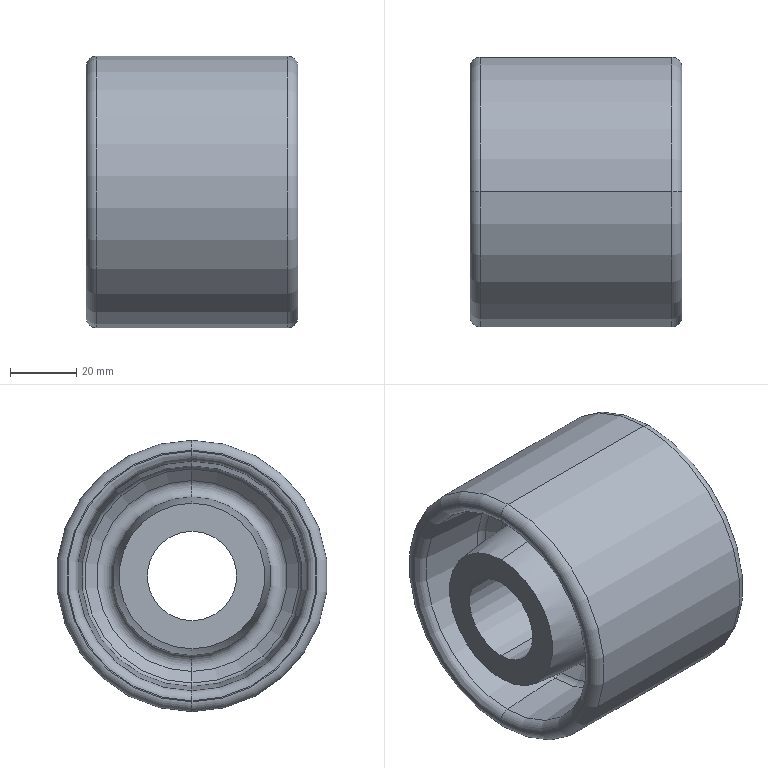Part | SolidWorks | features Revolution 1 | 1 solid | 36 faces | box 64 x 82 x 82 mm | volume 200004 mm3 | torus 24 | cone 4 | plane 4 | cylinder 4 | commonest cylinder face diameters 27 x2 82 x2
STEP:
#1=CARTESIAN_POINT('',(-32.713,0.,48.22));
#2=VERTEX_POINT('',#1);
#3=CARTESIAN_POINT('',(-32.713,0.,-21.22));
#4=VERTEX_POINT('',#3);
#5=CARTESIAN_POINT('',(-32.713,0.,13.5));
#6=DIRECTION('',(-1.,0.,0.));
#7=DIRECTION('',(0.,0.,1.));
#8=AXIS2_PLACEMENT_3D('',#5,#6,#7);
#9=CIRCLE('',#8,34.72);
#10=EDGE_CURVE('',#2,#4,#9,.T.);
#11=ORIENTED_EDGE('',*,*,#10,.T.);
#12=CARTESIAN_POINT('',(-12.328,0.,-19.908));
#13=VERTEX_POINT('',#12);
#14=CARTESIAN_POINT('',(-3.418,0.,-317.446));
#15=DIRECTION('',(0.,1.,0.));
#16=DIRECTION('',(0.,0.,1.));
#17=AXIS2_PLACEMENT_3D('',#14,#15,#16);
#18=CIRCLE('',#17,297.671);
#19=EDGE_CURVE('',#4,#13,#18,.T.);
#20=ORIENTED_EDGE('',*,*,#19,.T.);
#21=CARTESIAN_POINT('',(-12.328,0.,46.908));
#22=VERTEX_POINT('',#21);
#23=CARTESIAN_POINT('',(-12.328,0.,13.5));
#24=DIRECTION('',(-1.,0.,0.));
#25=DIRECTION('',(0.,0.,1.));
#26=AXIS2_PLACEMENT_3D('',#23,#24,#25);
#27=CIRCLE('',#26,33.408);
#28=EDGE_CURVE('',#22,#13,#27,.T.);
#29=ORIENTED_EDGE('',*,*,#28,.F.);
#30=CARTESIAN_POINT('',(-3.418,0.,344.446));
#31=DIRECTION('',(0.,-1.,0.));
#32=DIRECTION('',(0.,0.,-1.));
#33=AXIS2_PLACEMENT_3D('',#30,#31,#32);
#34=CIRCLE('',#33,297.671);
#35=EDGE_CURVE('',#2,#22,#34,.T.);
#36=ORIENTED_EDGE('',*,*,#35,.F.);
#37=EDGE_LOOP('',(#11,#20,#29,#36));
#38=FACE_OUTER_BOUND('',#37,.T.);
#39=CARTESIAN_POINT('',(-3.418,0.,13.5));
#40=DIRECTION('',(-1.,0.,0.));
#41=DIRECTION('',(0.,0.,1.));
#42=AXIS2_PLACEMENT_3D('',#39,#40,#41);
#43=TOROIDAL_SURFACE('',#42,330.946,297.671);
#44=ADVANCED_FACE('',(#38),#43,.T.);
#45=CARTESIAN_POINT('',(-35.418,0.,51.205));
#46=VERTEX_POINT('',#45);
#47=CARTESIAN_POINT('',(-35.418,0.,-24.205));
#48=VERTEX_POINT('',#47);
#49=CARTESIAN_POINT('',(-35.418,0.,13.5));
#50=DIRECTION('',(-1.,0.,0.));
#51=DIRECTION('',(0.,0.,1.));
#52=AXIS2_PLACEMENT_3D('',#49,#50,#51);
#53=CIRCLE('',#52,37.705);
#54=EDGE_CURVE('',#46,#48,#53,.T.);
#55=ORIENTED_EDGE('',*,*,#54,.T.);
#56=CARTESIAN_POINT('',(-32.418,0.,-24.205));
#57=DIRECTION('',(0.,1.,0.));
#58=DIRECTION('',(0.,0.,1.));
#59=AXIS2_PLACEMENT_3D('',#56,#57,#58);
#60=CIRCLE('',#59,3.);
#61=EDGE_CURVE('',#48,#4,#60,.T.);
#62=ORIENTED_EDGE('',*,*,#61,.T.);
#63=ORIENTED_EDGE('',*,*,#10,.F.);
#64=CARTESIAN_POINT('',(-32.418,0.,51.205));
#65=DIRECTION('',(0.,-1.,0.));
#66=DIRECTION('',(0.,0.,-1.));
#67=AXIS2_PLACEMENT_3D('',#64,#65,#66);
#68=CIRCLE('',#67,3.);
#69=EDGE_CURVE('',#46,#2,#68,.T.);
#70=ORIENTED_EDGE('',*,*,#69,.F.);
#71=EDGE_LOOP('',(#55,#62,#63,#70));
#72=FACE_OUTER_BOUND('',#71,.T.);
#73=CARTESIAN_POINT('',(-32.418,0.,13.5));
#74=DIRECTION('',(-1.,0.,0.));
#75=DIRECTION('',(0.,0.,1.));
#76=AXIS2_PLACEMENT_3D('',#73,#74,#75);
#77=TOROIDAL_SURFACE('',#76,37.705,3.);
#78=ADVANCED_FACE('',(#72),#77,.T.);
#79=CARTESIAN_POINT('',(-32.418,0.,54.5));
#80=VERTEX_POINT('',#79);
#81=CARTESIAN_POINT('',(-32.418,0.,-27.5));
#82=VERTEX_POINT('',#81);
#83=CARTESIAN_POINT('',(-32.418,0.,13.5));
#84=DIRECTION('',(-1.,0.,0.));
#85=DIRECTION('',(0.,0.,1.));
#86=AXIS2_PLACEMENT_3D('',#83,#84,#85);
#87=CIRCLE('',#86,41.);
#88=EDGE_CURVE('',#80,#82,#87,.T.);
#89=ORIENTED_EDGE('',*,*,#88,.T.);
#90=CARTESIAN_POINT('',(-35.418,0.,-24.5));
#91=VERTEX_POINT('',#90);
#92=CARTESIAN_POINT('',(-32.418,0.,-24.5));
#93=DIRECTION('',(0.,1.,0.));
#94=DIRECTION('',(0.,0.,1.));
#95=AXIS2_PLACEMENT_3D('',#92,#93,#94);
#96=CIRCLE('',#95,3.);
#97=EDGE_CURVE('',#82,#91,#96,.T.);
#98=ORIENTED_EDGE('',*,*,#97,.T.);
#99=CARTESIAN_POINT('',(-35.418,0.,51.5));
#100=VERTEX_POINT('',#99);
#101=CARTESIAN_POINT('',(-35.418,0.,13.5));
#102=DIRECTION('',(-1.,0.,0.));
#103=DIRECTION('',(0.,0.,1.));
#104=AXIS2_PLACEMENT_3D('',#101,#102,#103);
#105=CIRCLE('',#104,38.);
#106=EDGE_CURVE('',#100,#91,#105,.T.);
#107=ORIENTED_EDGE('',*,*,#106,.F.);
#108=CARTESIAN_POINT('',(-32.418,0.,51.5));
#109=DIRECTION('',(0.,-1.,0.));
#110=DIRECTION('',(0.,0.,-1.));
#111=AXIS2_PLACEMENT_3D('',#108,#109,#110);
#112=CIRCLE('',#111,3.);
#113=EDGE_CURVE('',#80,#100,#112,.T.);
#114=ORIENTED_EDGE('',*,*,#113,.F.);
#115=EDGE_LOOP('',(#89,#98,#107,#114));
#116=FACE_OUTER_BOUND('',#115,.T.);
#117=CARTESIAN_POINT('',(-32.418,0.,13.5));
#118=DIRECTION('',(-1.,0.,0.));
#119=DIRECTION('',(0.,0.,1.));
#120=AXIS2_PLACEMENT_3D('',#117,#118,#119);
#121=TOROIDAL_SURFACE('',#120,38.,3.);
#122=ADVANCED_FACE('',(#116),#121,.T.);
#123=CARTESIAN_POINT('',(25.582,0.,54.5));
#124=VERTEX_POINT('',#123);
#125=CARTESIAN_POINT('',(25.582,0.,-27.5));
#126=VERTEX_POINT('',#125);
#127=CARTESIAN_POINT('',(25.582,0.,13.5));
#128=DIRECTION('',(-1.,0.,0.));
#129=DIRECTION('',(0.,0.,1.));
#130=AXIS2_PLACEMENT_3D('',#127,#128,#129);
#131=CIRCLE('',#130,41.);
#132=EDGE_CURVE('',#124,#126,#131,.T.);
#133=ORIENTED_EDGE('',*,*,#132,.T.);
#134=CARTESIAN_POINT('',(-39.429,0.,-27.5));
#135=DIRECTION('',(-1.,0.,0.));
#136=VECTOR('',#135,1000.);
#137=LINE('',#134,#136);
#138=EDGE_CURVE('',#126,#82,#137,.T.);
#139=ORIENTED_EDGE('',*,*,#138,.T.);
#140=ORIENTED_EDGE('',*,*,#88,.F.);
#141=CARTESIAN_POINT('',(-39.429,0.,54.5));
#142=DIRECTION('',(-1.,0.,0.));
#143=VECTOR('',#142,1000.);
#144=LINE('',#141,#143);
#145=EDGE_CURVE('',#124,#80,#144,.T.);
#146=ORIENTED_EDGE('',*,*,#145,.F.);
#147=EDGE_LOOP('',(#133,#139,#140,#146));
#148=FACE_OUTER_BOUND('',#147,.T.);
#149=CARTESIAN_POINT('',(-39.429,0.,13.5));
#150=DIRECTION('',(-1.,0.,0.));
#151=DIRECTION('',(0.,0.,1.));
#152=AXIS2_PLACEMENT_3D('',#149,#150,#151);
#153=CYLINDRICAL_SURFACE('',#152,41.);
#154=ADVANCED_FACE('',(#148),#153,.T.);
#155=CARTESIAN_POINT('',(28.582,0.,51.5));
#156=VERTEX_POINT('',#155);
#157=CARTESIAN_POINT('',(28.582,0.,-24.5));
#158=VERTEX_POINT('',#157);
#159=CARTESIAN_POINT('',(28.582,0.,13.5));
#160=DIRECTION('',(-1.,0.,0.));
#161=DIRECTION('',(0.,0.,1.));
#162=AXIS2_PLACEMENT_3D('',#159,#160,#161);
#163=CIRCLE('',#162,38.);
#164=EDGE_CURVE('',#156,#158,#163,.T.);
#165=ORIENTED_EDGE('',*,*,#164,.T.);
#166=CARTESIAN_POINT('',(25.582,0.,-24.5));
#167=DIRECTION('',(0.,1.,0.));
#168=DIRECTION('',(0.,0.,1.));
#169=AXIS2_PLACEMENT_3D('',#166,#167,#168);
#170=CIRCLE('',#169,3.);
#171=EDGE_CURVE('',#158,#126,#170,.T.);
#172=ORIENTED_EDGE('',*,*,#171,.T.);
#173=ORIENTED_EDGE('',*,*,#132,.F.);
#174=CARTESIAN_POINT('',(25.582,0.,51.5));
#175=DIRECTION('',(0.,-1.,0.));
#176=DIRECTION('',(0.,0.,-1.));
#177=AXIS2_PLACEMENT_3D('',#174,#175,#176);
#178=CIRCLE('',#177,3.);
#179=EDGE_CURVE('',#156,#124,#178,.T.);
#180=ORIENTED_EDGE('',*,*,#179,.F.);
#181=EDGE_LOOP('',(#165,#172,#173,#180));
#182=FACE_OUTER_BOUND('',#181,.T.);
#183=CARTESIAN_POINT('',(25.582,0.,13.5));
#184=DIRECTION('',(-1.,0.,0.));
#185=DIRECTION('',(0.,0.,1.));
#186=AXIS2_PLACEMENT_3D('',#183,#184,#185);
#187=TOROIDAL_SURFACE('',#186,38.,3.);
#188=ADVANCED_FACE('',(#182),#187,.T.);
#189=CARTESIAN_POINT('',(25.877,0.,48.22));
#190=VERTEX_POINT('',#189);
#191=CARTESIAN_POINT('',(25.877,0.,-21.22));
#192=VERTEX_POINT('',#191);
#193=CARTESIAN_POINT('',(25.877,0.,13.5));
#194=DIRECTION('',(-1.,0.,0.));
#195=DIRECTION('',(0.,0.,1.));
#196=AXIS2_PLACEMENT_3D('',#193,#194,#195);
#197=CIRCLE('',#196,34.72);
#198=EDGE_CURVE('',#190,#192,#197,.T.);
#199=ORIENTED_EDGE('',*,*,#198,.T.);
#200=CARTESIAN_POINT('',(28.582,0.,-24.205));
#201=VERTEX_POINT('',#200);
#202=CARTESIAN_POINT('',(25.582,0.,-24.205));
#203=DIRECTION('',(0.,1.,0.));
#204=DIRECTION('',(0.,0.,1.));
#205=AXIS2_PLACEMENT_3D('',#202,#203,#204);
#206=CIRCLE('',#205,3.);
#207=EDGE_CURVE('',#192,#201,#206,.T.);
#208=ORIENTED_EDGE('',*,*,#207,.T.);
#209=CARTESIAN_POINT('',(28.582,0.,51.205));
#210=VERTEX_POINT('',#209);
#211=CARTESIAN_POINT('',(28.582,0.,13.5));
#212=DIRECTION('',(-1.,0.,0.));
#213=DIRECTION('',(0.,0.,1.));
#214=AXIS2_PLACEMENT_3D('',#211,#212,#213);
#215=CIRCLE('',#214,37.705);
#216=EDGE_CURVE('',#210,#201,#215,.T.);
#217=ORIENTED_EDGE('',*,*,#216,.F.);
#218=CARTESIAN_POINT('',(25.582,0.,51.205));
#219=DIRECTION('',(0.,-1.,0.));
#220=DIRECTION('',(0.,0.,-1.));
#221=AXIS2_PLACEMENT_3D('',#218,#219,#220);
#222=CIRCLE('',#221,3.);
#223=EDGE_CURVE('',#190,#210,#222,.T.);
#224=ORIENTED_EDGE('',*,*,#223,.F.);
#225=EDGE_LOOP('',(#199,#208,#217,#224));
#226=FACE_OUTER_BOUND('',#225,.T.);
#227=CARTESIAN_POINT('',(25.582,0.,13.5));
#228=DIRECTION('',(-1.,0.,0.));
#229=DIRECTION('',(0.,0.,1.));
#230=AXIS2_PLACEMENT_3D('',#227,#228,#229);
#231=TOROIDAL_SURFACE('',#230,37.705,3.);
#232=ADVANCED_FACE('',(#226),#231,.T.);
#233=CARTESIAN_POINT('',(5.492,0.,46.908));
#234=VERTEX_POINT('',#233);
#235=CARTESIAN_POINT('',(5.492,0.,-19.908));
#236=VERTEX_POINT('',#235);
#237=CARTESIAN_POINT('',(5.492,0.,13.5));
#238=DIRECTION('',(-1.,0.,0.));
#239=DIRECTION('',(0.,0.,1.));
#240=AXIS2_PLACEMENT_3D('',#237,#238,#239);
#241=CIRCLE('',#240,33.408);
#242=EDGE_CURVE('',#234,#236,#241,.T.);
#243=ORIENTED_EDGE('',*,*,#242,.T.);
#244=CARTESIAN_POINT('',(-3.418,0.,-317.446));
#245=DIRECTION('',(0.,1.,0.));
#246=DIRECTION('',(0.,0.,1.));
#247=AXIS2_PLACEMENT_3D('',#244,#245,#246);
#248=CIRCLE('',#247,297.671);
#249=EDGE_CURVE('',#236,#192,#248,.T.);
#250=ORIENTED_EDGE('',*,*,#249,.T.);
#251=ORIENTED_EDGE('',*,*,#198,.F.);
#252=CARTESIAN_POINT('',(-3.418,0.,344.446));
#253=DIRECTION('',(0.,-1.,0.));
#254=DIRECTION('',(0.,0.,-1.));
#255=AXIS2_PLACEMENT_3D('',#252,#253,#254);
#256=CIRCLE('',#255,297.671);
#257=EDGE_CURVE('',#234,#190,#256,.T.);
#258=ORIENTED_EDGE('',*,*,#257,.F.);
#259=EDGE_LOOP('',(#243,#250,#251,#258));
#260=FACE_OUTER_BOUND('',#259,.T.);
#261=CARTESIAN_POINT('',(-3.418,0.,13.5));
#262=DIRECTION('',(-1.,0.,0.));
#263=DIRECTION('',(0.,0.,1.));
#264=AXIS2_PLACEMENT_3D('',#261,#262,#263);
#265=TOROIDAL_SURFACE('',#264,330.946,297.671);
#266=ADVANCED_FACE('',(#260),#265,.T.);
#267=CARTESIAN_POINT('',(5.492,0.,13.5));
#268=DIRECTION('',(-1.,0.,0.));
#269=DIRECTION('',(0.,0.,1.));
#270=AXIS2_PLACEMENT_3D('',#267,#268,#269);
#271=CIRCLE('',#270,33.408);
#272=EDGE_CURVE('',#236,#234,#271,.T.);
#273=ORIENTED_EDGE('',*,*,#272,.F.);
#274=CARTESIAN_POINT('',(3.298,0.,-14.965));
#275=VERTEX_POINT('',#274);
#276=CARTESIAN_POINT('',(5.582,0.,-16.91));
#277=DIRECTION('',(0.,1.,0.));
#278=DIRECTION('',(0.,0.,1.));
#279=AXIS2_PLACEMENT_3D('',#276,#277,#278);
#280=CIRCLE('',#279,3.);
#281=EDGE_CURVE('',#236,#275,#280,.T.);
#282=ORIENTED_EDGE('',*,*,#281,.T.);
#283=CARTESIAN_POINT('',(3.298,0.,41.965));
#284=VERTEX_POINT('',#283);
#285=CARTESIAN_POINT('',(3.298,0.,13.5));
#286=DIRECTION('',(-1.,0.,0.));
#287=DIRECTION('',(0.,0.,1.));
#288=AXIS2_PLACEMENT_3D('',#285,#286,#287);
#289=CIRCLE('',#288,28.465);
#290=EDGE_CURVE('',#275,#284,#289,.T.);
#291=ORIENTED_EDGE('',*,*,#290,.T.);
#292=CARTESIAN_POINT('',(5.582,0.,43.91));
#293=DIRECTION('',(0.,-1.,0.));
#294=DIRECTION('',(0.,0.,-1.));
#295=AXIS2_PLACEMENT_3D('',#292,#293,#294);
#296=CIRCLE('',#295,3.);
#297=EDGE_CURVE('',#234,#284,#296,.T.);
#298=ORIENTED_EDGE('',*,*,#297,.F.);
#299=EDGE_LOOP('',(#273,#282,#291,#298));
#300=FACE_OUTER_BOUND('',#299,.T.);
#301=CARTESIAN_POINT('',(5.582,0.,13.5));
#302=DIRECTION('',(-1.,0.,0.));
#303=DIRECTION('',(0.,0.,1.));
#304=AXIS2_PLACEMENT_3D('',#301,#302,#303);
#305=TOROIDAL_SURFACE('',#304,30.41,3.);
#306=ADVANCED_FACE('',(#300),#305,.F.);
#307=CARTESIAN_POINT('',(6.298,0.,38.442));
#308=VERTEX_POINT('',#307);
#309=CARTESIAN_POINT('',(6.298,0.,-11.442));
#310=VERTEX_POINT('',#309);
#311=CARTESIAN_POINT('',(6.298,0.,13.5));
#312=DIRECTION('',(-1.,0.,0.));
#313=DIRECTION('',(0.,0.,1.));
#314=AXIS2_PLACEMENT_3D('',#311,#312,#313);
#315=CIRCLE('',#314,24.942);
#316=EDGE_CURVE('',#308,#310,#315,.T.);
#317=ORIENTED_EDGE('',*,*,#316,.T.);
#318=CARTESIAN_POINT('',(6.298,0.,-11.442));
#319=DIRECTION('',(-0.6484,0.,-0.7613));
#320=VECTOR('',#319,1000.);
#321=LINE('',#318,#320);
#322=EDGE_CURVE('',#310,#275,#321,.T.);
#323=ORIENTED_EDGE('',*,*,#322,.T.);
#324=CARTESIAN_POINT('',(3.298,0.,13.5));
#325=DIRECTION('',(-1.,0.,0.));
#326=DIRECTION('',(0.,0.,1.));
#327=AXIS2_PLACEMENT_3D('',#324,#325,#326);
#328=CIRCLE('',#327,28.465);
#329=EDGE_CURVE('',#284,#275,#328,.T.);
#330=ORIENTED_EDGE('',*,*,#329,.F.);
#331=CARTESIAN_POINT('',(6.298,0.,38.442));
#332=DIRECTION('',(-0.6484,0.,0.7613));
#333=VECTOR('',#332,1000.);
#334=LINE('',#331,#333);
#335=EDGE_CURVE('',#308,#284,#334,.T.);
#336=ORIENTED_EDGE('',*,*,#335,.F.);
#337=EDGE_LOOP('',(#317,#323,#330,#336));
#338=FACE_OUTER_BOUND('',#337,.T.);
#339=CARTESIAN_POINT('',(6.298,0.,13.5));
#340=DIRECTION('',(-1.,0.,0.));
#341=DIRECTION('',(0.,0.,1.));
#342=AXIS2_PLACEMENT_3D('',#339,#340,#341);
#343=CONICAL_SURFACE('',#342,24.942,0.8653);
#344=ADVANCED_FACE('',(#338),#343,.T.);
#345=CARTESIAN_POINT('',(6.298,0.,13.5));
#346=DIRECTION('',(-1.,0.,0.));
#347=DIRECTION('',(0.,0.,1.));
#348=AXIS2_PLACEMENT_3D('',#345,#346,#347);
#349=CIRCLE('',#348,24.942);
#350=EDGE_CURVE('',#310,#308,#349,.T.);
#351=ORIENTED_EDGE('',*,*,#350,.F.);
#352=CARTESIAN_POINT('',(8.494,0.,-10.388));
#353=VERTEX_POINT('',#352);
#354=CARTESIAN_POINT('',(8.582,0.,-13.387));
#355=DIRECTION('',(0.,1.,0.));
#356=DIRECTION('',(0.,0.,1.));
#357=AXIS2_PLACEMENT_3D('',#354,#355,#356);
#358=CIRCLE('',#357,3.);
#359=EDGE_CURVE('',#310,#353,#358,.T.);
#360=ORIENTED_EDGE('',*,*,#359,.T.);
#361=CARTESIAN_POINT('',(8.494,0.,37.388));
#362=VERTEX_POINT('',#361);
#363=CARTESIAN_POINT('',(8.494,0.,13.5));
#364=DIRECTION('',(-1.,0.,0.));
#365=DIRECTION('',(0.,0.,1.));
#366=AXIS2_PLACEMENT_3D('',#363,#364,#365);
#367=CIRCLE('',#366,23.888);
#368=EDGE_CURVE('',#353,#362,#367,.T.);
#369=ORIENTED_EDGE('',*,*,#368,.T.);
#370=CARTESIAN_POINT('',(8.582,0.,40.387));
#371=DIRECTION('',(0.,-1.,0.));
#372=DIRECTION('',(0.,0.,-1.));
#373=AXIS2_PLACEMENT_3D('',#370,#371,#372);
#374=CIRCLE('',#373,3.);
#375=EDGE_CURVE('',#308,#362,#374,.T.);
#376=ORIENTED_EDGE('',*,*,#375,.F.);
#377=EDGE_LOOP('',(#351,#360,#369,#376));
#378=FACE_OUTER_BOUND('',#377,.T.);
#379=CARTESIAN_POINT('',(8.582,0.,13.5));
#380=DIRECTION('',(-1.,0.,0.));
#381=DIRECTION('',(0.,0.,1.));
#382=AXIS2_PLACEMENT_3D('',#379,#380,#381);
#383=TOROIDAL_SURFACE('',#382,26.887,3.);
#384=ADVANCED_FACE('',(#378),#383,.F.);
#385=CARTESIAN_POINT('',(28.582,0.,36.134));
#386=VERTEX_POINT('',#385);
#387=CARTESIAN_POINT('',(28.582,0.,-9.134));
#388=VERTEX_POINT('',#387);
#389=CARTESIAN_POINT('',(28.582,0.,13.5));
#390=DIRECTION('',(-1.,0.,0.));
#391=DIRECTION('',(0.,0.,1.));
#392=AXIS2_PLACEMENT_3D('',#389,#390,#391);
#393=CIRCLE('',#392,22.634);
#394=EDGE_CURVE('',#386,#388,#393,.T.);
#395=ORIENTED_EDGE('',*,*,#394,.T.);
#396=CARTESIAN_POINT('',(-0.4182,0.,293.862));
#397=DIRECTION('',(0.,1.,0.));
#398=DIRECTION('',(0.,0.,1.));
#399=AXIS2_PLACEMENT_3D('',#396,#397,#398);
#400=CIRCLE('',#399,304.381);
#401=EDGE_CURVE('',#388,#353,#400,.T.);
#402=ORIENTED_EDGE('',*,*,#401,.T.);
#403=CARTESIAN_POINT('',(8.494,0.,13.5));
#404=DIRECTION('',(-1.,0.,0.));
#405=DIRECTION('',(0.,0.,1.));
#406=AXIS2_PLACEMENT_3D('',#403,#404,#405);
#407=CIRCLE('',#406,23.888);
#408=EDGE_CURVE('',#362,#353,#407,.T.);
#409=ORIENTED_EDGE('',*,*,#408,.F.);
#410=CARTESIAN_POINT('',(-0.4182,0.,-266.862));
#411=DIRECTION('',(0.,-1.,0.));
#412=DIRECTION('',(0.,0.,-1.));
#413=AXIS2_PLACEMENT_3D('',#410,#411,#412);
#414=CIRCLE('',#413,304.381);
#415=EDGE_CURVE('',#386,#362,#414,.T.);
#416=ORIENTED_EDGE('',*,*,#415,.F.);
#417=EDGE_LOOP('',(#395,#402,#409,#416));
#418=FACE_OUTER_BOUND('',#417,.T.);
#419=CARTESIAN_POINT('',(-0.4182,0.,13.5));
#420=DIRECTION('',(-1.,0.,0.));
#421=DIRECTION('',(0.,0.,1.));
#422=AXIS2_PLACEMENT_3D('',#419,#420,#421);
#423=TOROIDAL_SURFACE('',#422,-280.362,304.381);
#424=ADVANCED_FACE('',(#418),#423,.T.);
#425=CARTESIAN_POINT('',(28.582,0.,0.));
#426=VERTEX_POINT('',#425);
#427=CARTESIAN_POINT('',(28.582,0.,27.));
#428=VERTEX_POINT('',#427);
#429=CARTESIAN_POINT('',(28.582,0.,13.5));
#430=DIRECTION('',(-1.,0.,0.));
#431=DIRECTION('',(0.,0.,1.));
#432=AXIS2_PLACEMENT_3D('',#429,#430,#431);
#433=CIRCLE('',#432,13.5);
#434=EDGE_CURVE('',#426,#428,#433,.T.);
#435=ORIENTED_EDGE('',*,*,#434,.F.);
#436=CARTESIAN_POINT('',(-35.418,0.,0.));
#437=VERTEX_POINT('',#436);
#438=CARTESIAN_POINT('',(-39.429,0.,0.));
#439=DIRECTION('',(-1.,0.,0.));
#440=VECTOR('',#439,1000.);
#441=LINE('',#438,#440);
#442=EDGE_CURVE('',#426,#437,#441,.T.);
#443=ORIENTED_EDGE('',*,*,#442,.T.);
#444=CARTESIAN_POINT('',(-35.418,0.,27.));
#445=VERTEX_POINT('',#444);
#446=CARTESIAN_POINT('',(-35.418,0.,13.5));
#447=DIRECTION('',(-1.,0.,0.));
#448=DIRECTION('',(0.,0.,1.));
#449=AXIS2_PLACEMENT_3D('',#446,#447,#448);
#450=CIRCLE('',#449,13.5);
#451=EDGE_CURVE('',#437,#445,#450,.T.);
#452=ORIENTED_EDGE('',*,*,#451,.T.);
#453=CARTESIAN_POINT('',(-39.429,0.,27.));
#454=DIRECTION('',(-1.,0.,0.));
#455=VECTOR('',#454,1000.);
#456=LINE('',#453,#455);
#457=EDGE_CURVE('',#428,#445,#456,.T.);
#458=ORIENTED_EDGE('',*,*,#457,.F.);
#459=EDGE_LOOP('',(#435,#443,#452,#458));
#460=FACE_OUTER_BOUND('',#459,.T.);
#461=CARTESIAN_POINT('',(-39.429,0.,13.5));
#462=DIRECTION('',(-1.,0.,0.));
#463=DIRECTION('',(0.,0.,1.));
#464=AXIS2_PLACEMENT_3D('',#461,#462,#463);
#465=CYLINDRICAL_SURFACE('',#464,13.5);
#466=ADVANCED_FACE('',(#460),#465,.F.);
#467=CARTESIAN_POINT('',(-9.33,0.,37.388));
#468=VERTEX_POINT('',#467);
#469=CARTESIAN_POINT('',(-9.33,0.,-10.388));
#470=VERTEX_POINT('',#469);
#471=CARTESIAN_POINT('',(-9.33,0.,13.5));
#472=DIRECTION('',(-1.,0.,0.));
#473=DIRECTION('',(0.,0.,1.));
#474=AXIS2_PLACEMENT_3D('',#471,#472,#473);
#475=CIRCLE('',#474,23.888);
#476=EDGE_CURVE('',#468,#470,#475,.T.);
#477=ORIENTED_EDGE('',*,*,#476,.T.);
#478=CARTESIAN_POINT('',(-35.418,0.,-8.5));
#479=VERTEX_POINT('',#478);
#480=CARTESIAN_POINT('',(-0.4182,0.,293.862));
#481=DIRECTION('',(0.,1.,0.));
#482=DIRECTION('',(0.,0.,1.));
#483=AXIS2_PLACEMENT_3D('',#480,#481,#482);
#484=CIRCLE('',#483,304.381);
#485=EDGE_CURVE('',#470,#479,#484,.T.);
#486=ORIENTED_EDGE('',*,*,#485,.T.);
#487=CARTESIAN_POINT('',(-35.418,0.,35.5));
#488=VERTEX_POINT('',#487);
#489=CARTESIAN_POINT('',(-35.418,0.,13.5));
#490=DIRECTION('',(-1.,0.,0.));
#491=DIRECTION('',(0.,0.,1.));
#492=AXIS2_PLACEMENT_3D('',#489,#490,#491);
#493=CIRCLE('',#492,22.);
#494=EDGE_CURVE('',#488,#479,#493,.T.);
#495=ORIENTED_EDGE('',*,*,#494,.F.);
#496=CARTESIAN_POINT('',(-0.4182,0.,-266.862));
#497=DIRECTION('',(0.,-1.,0.));
#498=DIRECTION('',(0.,0.,-1.));
#499=AXIS2_PLACEMENT_3D('',#496,#497,#498);
#500=CIRCLE('',#499,304.381);
#501=EDGE_CURVE('',#468,#488,#500,.T.);
#502=ORIENTED_EDGE('',*,*,#501,.F.);
#503=EDGE_LOOP('',(#477,#486,#495,#502));
#504=FACE_OUTER_BOUND('',#503,.T.);
#505=CARTESIAN_POINT('',(-0.4182,0.,13.5));
#506=DIRECTION('',(-1.,0.,0.));
#507=DIRECTION('',(0.,0.,1.));
#508=AXIS2_PLACEMENT_3D('',#505,#506,#507);
#509=TOROIDAL_SURFACE('',#508,-280.362,304.381);
#510=ADVANCED_FACE('',(#504),#509,.T.);
#511=CARTESIAN_POINT('',(-9.33,0.,13.5));
#512=DIRECTION('',(-1.,0.,0.));
#513=DIRECTION('',(0.,0.,1.));
#514=AXIS2_PLACEMENT_3D('',#511,#512,#513);
#515=CIRCLE('',#514,23.888);
#516=EDGE_CURVE('',#470,#468,#515,.T.);
#517=ORIENTED_EDGE('',*,*,#516,.F.);
#518=CARTESIAN_POINT('',(-7.134,0.,-15.332));
#519=VERTEX_POINT('',#518);
#520=CARTESIAN_POINT('',(-9.418,0.,-13.387));
#521=DIRECTION('',(0.,1.,0.));
#522=DIRECTION('',(0.,0.,1.));
#523=AXIS2_PLACEMENT_3D('',#520,#521,#522);
#524=CIRCLE('',#523,3.);
#525=EDGE_CURVE('',#470,#519,#524,.T.);
#526=ORIENTED_EDGE('',*,*,#525,.T.);
#527=CARTESIAN_POINT('',(-7.134,0.,42.332));
#528=VERTEX_POINT('',#527);
#529=CARTESIAN_POINT('',(-7.134,0.,13.5));
#530=DIRECTION('',(-1.,0.,0.));
#531=DIRECTION('',(0.,0.,1.));
#532=AXIS2_PLACEMENT_3D('',#529,#530,#531);
#533=CIRCLE('',#532,28.832);
#534=EDGE_CURVE('',#519,#528,#533,.T.);
#535=ORIENTED_EDGE('',*,*,#534,.T.);
#536=CARTESIAN_POINT('',(-9.418,0.,40.387));
#537=DIRECTION('',(0.,-1.,0.));
#538=DIRECTION('',(0.,0.,-1.));
#539=AXIS2_PLACEMENT_3D('',#536,#537,#538);
#540=CIRCLE('',#539,3.);
#541=EDGE_CURVE('',#468,#528,#540,.T.);
#542=ORIENTED_EDGE('',*,*,#541,.F.);
#543=EDGE_LOOP('',(#517,#526,#535,#542));
#544=FACE_OUTER_BOUND('',#543,.T.);
#545=CARTESIAN_POINT('',(-9.418,0.,13.5));
#546=DIRECTION('',(-1.,0.,0.));
#547=DIRECTION('',(0.,0.,1.));
#548=AXIS2_PLACEMENT_3D('',#545,#546,#547);
#549=TOROIDAL_SURFACE('',#548,26.887,3.);
#550=ADVANCED_FACE('',(#544),#549,.F.);
#551=ORIENTED_EDGE('',*,*,#534,.F.);
#552=CARTESIAN_POINT('',(-10.134,0.,-18.855));
#553=VERTEX_POINT('',#552);
#554=CARTESIAN_POINT('',(-10.134,0.,-18.855));
#555=DIRECTION('',(-0.6484,0.,-0.7613));
#556=VECTOR('',#555,1000.);
#557=LINE('',#554,#556);
#558=EDGE_CURVE('',#519,#553,#557,.T.);
#559=ORIENTED_EDGE('',*,*,#558,.T.);
#560=CARTESIAN_POINT('',(-10.134,0.,45.855));
#561=VERTEX_POINT('',#560);
#562=CARTESIAN_POINT('',(-10.134,0.,13.5));
#563=DIRECTION('',(-1.,0.,0.));
#564=DIRECTION('',(0.,0.,1.));
#565=AXIS2_PLACEMENT_3D('',#562,#563,#564);
#566=CIRCLE('',#565,32.355);
#567=EDGE_CURVE('',#553,#561,#566,.T.);
#568=ORIENTED_EDGE('',*,*,#567,.T.);
#569=CARTESIAN_POINT('',(-10.134,0.,45.855));
#570=DIRECTION('',(-0.6484,0.,0.7613));
#571=VECTOR('',#570,1000.);
#572=LINE('',#569,#571);
#573=EDGE_CURVE('',#528,#561,#572,.T.);
#574=ORIENTED_EDGE('',*,*,#573,.F.);
#575=EDGE_LOOP('',(#551,#559,#568,#574));
#576=FACE_OUTER_BOUND('',#575,.T.);
#577=CARTESIAN_POINT('',(-10.134,0.,13.5));
#578=DIRECTION('',(-1.,0.,0.));
#579=DIRECTION('',(0.,0.,1.));
#580=AXIS2_PLACEMENT_3D('',#577,#578,#579);
#581=CONICAL_SURFACE('',#580,32.355,0.8653);
#582=ADVANCED_FACE('',(#576),#581,.F.);
#583=ORIENTED_EDGE('',*,*,#567,.F.);
#584=CARTESIAN_POINT('',(-12.418,0.,-16.91));
#585=DIRECTION('',(0.,1.,0.));
#586=DIRECTION('',(0.,0.,1.));
#587=AXIS2_PLACEMENT_3D('',#584,#585,#586);
#588=CIRCLE('',#587,3.);
#589=EDGE_CURVE('',#553,#13,#588,.T.);
#590=ORIENTED_EDGE('',*,*,#589,.T.);
#591=CARTESIAN_POINT('',(-12.328,0.,13.5));
#592=DIRECTION('',(-1.,0.,0.));
#593=DIRECTION('',(0.,0.,1.));
#594=AXIS2_PLACEMENT_3D('',#591,#592,#593);
#595=CIRCLE('',#594,33.408);
#596=EDGE_CURVE('',#13,#22,#595,.T.);
#597=ORIENTED_EDGE('',*,*,#596,.T.);
#598=CARTESIAN_POINT('',(-12.418,0.,43.91));
#599=DIRECTION('',(0.,-1.,0.));
#600=DIRECTION('',(0.,0.,-1.));
#601=AXIS2_PLACEMENT_3D('',#598,#599,#600);
#602=CIRCLE('',#601,3.);
#603=EDGE_CURVE('',#561,#22,#602,.T.);
#604=ORIENTED_EDGE('',*,*,#603,.F.);
#605=EDGE_LOOP('',(#583,#590,#597,#604));
#606=FACE_OUTER_BOUND('',#605,.T.);
#607=CARTESIAN_POINT('',(-12.418,0.,13.5));
#608=DIRECTION('',(-1.,0.,0.));
#609=DIRECTION('',(0.,0.,1.));
#610=AXIS2_PLACEMENT_3D('',#607,#608,#609);
#611=TOROIDAL_SURFACE('',#610,30.41,3.);
#612=ADVANCED_FACE('',(#606),#611,.F.);
#613=ORIENTED_EDGE('',*,*,#589,.F.);
#614=CARTESIAN_POINT('',(-10.134,0.,13.5));
#615=DIRECTION('',(-1.,0.,0.));
#616=DIRECTION('',(0.,0.,1.));
#617=AXIS2_PLACEMENT_3D('',#614,#615,#616);
#618=CIRCLE('',#617,32.355);
#619=EDGE_CURVE('',#561,#553,#618,.T.);
#620=ORIENTED_EDGE('',*,*,#619,.F.);
#621=ORIENTED_EDGE('',*,*,#603,.T.);
#622=ORIENTED_EDGE('',*,*,#28,.T.);
#623=EDGE_LOOP('',(#613,#620,#621,#622));
#624=FACE_OUTER_BOUND('',#623,.T.);
#625=CARTESIAN_POINT('',(-12.418,0.,13.5));
#626=DIRECTION('',(-1.,0.,0.));
#627=DIRECTION('',(0.,0.,1.));
#628=AXIS2_PLACEMENT_3D('',#625,#626,#627);
#629=TOROIDAL_SURFACE('',#628,30.41,3.);
#630=ADVANCED_FACE('',(#624),#629,.F.);
#631=ORIENTED_EDGE('',*,*,#558,.F.);
#632=CARTESIAN_POINT('',(-7.134,0.,13.5));
#633=DIRECTION('',(-1.,0.,0.));
#634=DIRECTION('',(0.,0.,1.));
#635=AXIS2_PLACEMENT_3D('',#632,#633,#634);
#636=CIRCLE('',#635,28.832);
#637=EDGE_CURVE('',#528,#519,#636,.T.);
#638=ORIENTED_EDGE('',*,*,#637,.F.);
#639=ORIENTED_EDGE('',*,*,#573,.T.);
#640=ORIENTED_EDGE('',*,*,#619,.T.);
#641=EDGE_LOOP('',(#631,#638,#639,#640));
#642=FACE_OUTER_BOUND('',#641,.T.);
#643=CARTESIAN_POINT('',(-10.134,0.,13.5));
#644=DIRECTION('',(-1.,0.,0.));
#645=DIRECTION('',(0.,0.,1.));
#646=AXIS2_PLACEMENT_3D('',#643,#644,#645);
#647=CONICAL_SURFACE('',#646,32.355,0.8653);
#648=ADVANCED_FACE('',(#642),#647,.F.);
#649=ORIENTED_EDGE('',*,*,#525,.F.);
#650=ORIENTED_EDGE('',*,*,#476,.F.);
#651=ORIENTED_EDGE('',*,*,#541,.T.);
#652=ORIENTED_EDGE('',*,*,#637,.T.);
#653=EDGE_LOOP('',(#649,#650,#651,#652));
#654=FACE_OUTER_BOUND('',#653,.T.);
#655=CARTESIAN_POINT('',(-9.418,0.,13.5));
#656=DIRECTION('',(-1.,0.,0.));
#657=DIRECTION('',(0.,0.,1.));
#658=AXIS2_PLACEMENT_3D('',#655,#656,#657);
#659=TOROIDAL_SURFACE('',#658,26.887,3.);
#660=ADVANCED_FACE('',(#654),#659,.F.);
#661=ORIENTED_EDGE('',*,*,#485,.F.);
#662=ORIENTED_EDGE('',*,*,#516,.T.);
#663=ORIENTED_EDGE('',*,*,#501,.T.);
#664=CARTESIAN_POINT('',(-35.418,0.,13.5));
#665=DIRECTION('',(-1.,0.,0.));
#666=DIRECTION('',(0.,0.,1.));
#667=AXIS2_PLACEMENT_3D('',#664,#665,#666);
#668=CIRCLE('',#667,22.);
#669=EDGE_CURVE('',#479,#488,#668,.T.);
#670=ORIENTED_EDGE('',*,*,#669,.F.);
#671=EDGE_LOOP('',(#661,#662,#663,#670));
#672=FACE_OUTER_BOUND('',#671,.T.);
#673=CARTESIAN_POINT('',(-0.4182,0.,13.5));
#674=DIRECTION('',(-1.,0.,0.));
#675=DIRECTION('',(0.,0.,1.));
#676=AXIS2_PLACEMENT_3D('',#673,#674,#675);
#677=TOROIDAL_SURFACE('',#676,-280.362,304.381);
#678=ADVANCED_FACE('',(#672),#677,.T.);
#679=CARTESIAN_POINT('',(-35.418,0.,13.5));
#680=DIRECTION('',(-1.,0.,0.));
#681=DIRECTION('',(0.,0.,1.));
#682=AXIS2_PLACEMENT_3D('',#679,#680,#681);
#683=CIRCLE('',#682,13.5);
#684=EDGE_CURVE('',#445,#437,#683,.T.);
#685=ORIENTED_EDGE('',*,*,#684,.F.);
#686=ORIENTED_EDGE('',*,*,#451,.F.);
#687=EDGE_LOOP('',(#685,#686));
#688=FACE_BOUND('',#687,.T.);
#689=ORIENTED_EDGE('',*,*,#494,.T.);
#690=ORIENTED_EDGE('',*,*,#669,.T.);
#691=EDGE_LOOP('',(#689,#690));
#692=FACE_OUTER_BOUND('',#691,.T.);
#693=CARTESIAN_POINT('',(-35.418,0.,-3.));
#694=DIRECTION('',(1.,0.,0.));
#695=DIRECTION('',(0.,0.,-1.));
#696=AXIS2_PLACEMENT_3D('',#693,#694,#695);
#697=PLANE('',#696);
#698=ADVANCED_FACE('',(#688,#692),#697,.F.);
#699=ORIENTED_EDGE('',*,*,#442,.F.);
#700=CARTESIAN_POINT('',(28.582,0.,13.5));
#701=DIRECTION('',(-1.,0.,0.));
#702=DIRECTION('',(0.,0.,1.));
#703=AXIS2_PLACEMENT_3D('',#700,#701,#702);
#704=CIRCLE('',#703,13.5);
#705=EDGE_CURVE('',#428,#426,#704,.T.);
#706=ORIENTED_EDGE('',*,*,#705,.F.);
#707=ORIENTED_EDGE('',*,*,#457,.T.);
#708=ORIENTED_EDGE('',*,*,#684,.T.);
#709=EDGE_LOOP('',(#699,#706,#707,#708));
#710=FACE_OUTER_BOUND('',#709,.T.);
#711=CARTESIAN_POINT('',(-39.429,0.,13.5));
#712=DIRECTION('',(-1.,0.,0.));
#713=DIRECTION('',(0.,0.,1.));
#714=AXIS2_PLACEMENT_3D('',#711,#712,#713);
#715=CYLINDRICAL_SURFACE('',#714,13.5);
#716=ADVANCED_FACE('',(#710),#715,.F.);
#717=ORIENTED_EDGE('',*,*,#394,.F.);
#718=CARTESIAN_POINT('',(28.582,0.,13.5));
#719=DIRECTION('',(-1.,0.,0.));
#720=DIRECTION('',(0.,0.,1.));
#721=AXIS2_PLACEMENT_3D('',#718,#719,#720);
#722=CIRCLE('',#721,22.634);
#723=EDGE_CURVE('',#388,#386,#722,.T.);
#724=ORIENTED_EDGE('',*,*,#723,.F.);
#725=EDGE_LOOP('',(#717,#724));
#726=FACE_OUTER_BOUND('',#725,.T.);
#727=ORIENTED_EDGE('',*,*,#705,.T.);
#728=ORIENTED_EDGE('',*,*,#434,.T.);
#729=EDGE_LOOP('',(#727,#728));
#730=FACE_BOUND('',#729,.T.);
#731=CARTESIAN_POINT('',(28.582,0.,-5.815));
#732=DIRECTION('',(-1.,0.,0.));
#733=DIRECTION('',(0.,0.,1.));
#734=AXIS2_PLACEMENT_3D('',#731,#732,#733);
#735=PLANE('',#734);
#736=ADVANCED_FACE('',(#726,#730),#735,.F.);
#737=ORIENTED_EDGE('',*,*,#401,.F.);
#738=ORIENTED_EDGE('',*,*,#723,.T.);
#739=ORIENTED_EDGE('',*,*,#415,.T.);
#740=ORIENTED_EDGE('',*,*,#368,.F.);
#741=EDGE_LOOP('',(#737,#738,#739,#740));
#742=FACE_OUTER_BOUND('',#741,.T.);
#743=CARTESIAN_POINT('',(-0.4182,0.,13.5));
#744=DIRECTION('',(-1.,0.,0.));
#745=DIRECTION('',(0.,0.,1.));
#746=AXIS2_PLACEMENT_3D('',#743,#744,#745);
#747=TOROIDAL_SURFACE('',#746,-280.362,304.381);
#748=ADVANCED_FACE('',(#742),#747,.T.);
#749=ORIENTED_EDGE('',*,*,#359,.F.);
#750=ORIENTED_EDGE('',*,*,#316,.F.);
#751=ORIENTED_EDGE('',*,*,#375,.T.);
#752=ORIENTED_EDGE('',*,*,#408,.T.);
#753=EDGE_LOOP('',(#749,#750,#751,#752));
#754=FACE_OUTER_BOUND('',#753,.T.);
#755=CARTESIAN_POINT('',(8.582,0.,13.5));
#756=DIRECTION('',(-1.,0.,0.));
#757=DIRECTION('',(0.,0.,1.));
#758=AXIS2_PLACEMENT_3D('',#755,#756,#757);
#759=TOROIDAL_SURFACE('',#758,26.887,3.);
#760=ADVANCED_FACE('',(#754),#759,.F.);
#761=ORIENTED_EDGE('',*,*,#322,.F.);
#762=ORIENTED_EDGE('',*,*,#350,.T.);
#763=ORIENTED_EDGE('',*,*,#335,.T.);
#764=ORIENTED_EDGE('',*,*,#290,.F.);
#765=EDGE_LOOP('',(#761,#762,#763,#764));
#766=FACE_OUTER_BOUND('',#765,.T.);
#767=CARTESIAN_POINT('',(6.298,0.,13.5));
#768=DIRECTION('',(-1.,0.,0.));
#769=DIRECTION('',(0.,0.,1.));
#770=AXIS2_PLACEMENT_3D('',#767,#768,#769);
#771=CONICAL_SURFACE('',#770,24.942,0.8653);
#772=ADVANCED_FACE('',(#766),#771,.T.);
#773=ORIENTED_EDGE('',*,*,#281,.F.);
#774=ORIENTED_EDGE('',*,*,#242,.F.);
#775=ORIENTED_EDGE('',*,*,#297,.T.);
#776=ORIENTED_EDGE('',*,*,#329,.T.);
#777=EDGE_LOOP('',(#773,#774,#775,#776));
#778=FACE_OUTER_BOUND('',#777,.T.);
#779=CARTESIAN_POINT('',(5.582,0.,13.5));
#780=DIRECTION('',(-1.,0.,0.));
#781=DIRECTION('',(0.,0.,1.));
#782=AXIS2_PLACEMENT_3D('',#779,#780,#781);
#783=TOROIDAL_SURFACE('',#782,30.41,3.);
#784=ADVANCED_FACE('',(#778),#783,.F.);
#785=ORIENTED_EDGE('',*,*,#249,.F.);
#786=ORIENTED_EDGE('',*,*,#272,.T.);
#787=ORIENTED_EDGE('',*,*,#257,.T.);
#788=CARTESIAN_POINT('',(25.877,0.,13.5));
#789=DIRECTION('',(-1.,0.,0.));
#790=DIRECTION('',(0.,0.,1.));
#791=AXIS2_PLACEMENT_3D('',#788,#789,#790);
#792=CIRCLE('',#791,34.72);
#793=EDGE_CURVE('',#192,#190,#792,.T.);
#794=ORIENTED_EDGE('',*,*,#793,.F.);
#795=EDGE_LOOP('',(#785,#786,#787,#794));
#796=FACE_OUTER_BOUND('',#795,.T.);
#797=CARTESIAN_POINT('',(-3.418,0.,13.5));
#798=DIRECTION('',(-1.,0.,0.));
#799=DIRECTION('',(0.,0.,1.));
#800=AXIS2_PLACEMENT_3D('',#797,#798,#799);
#801=TOROIDAL_SURFACE('',#800,330.946,297.671);
#802=ADVANCED_FACE('',(#796),#801,.T.);
#803=ORIENTED_EDGE('',*,*,#207,.F.);
#804=ORIENTED_EDGE('',*,*,#793,.T.);
#805=ORIENTED_EDGE('',*,*,#223,.T.);
#806=CARTESIAN_POINT('',(28.582,0.,13.5));
#807=DIRECTION('',(-1.,0.,0.));
#808=DIRECTION('',(0.,0.,1.));
#809=AXIS2_PLACEMENT_3D('',#806,#807,#808);
#810=CIRCLE('',#809,37.705);
#811=EDGE_CURVE('',#201,#210,#810,.T.);
#812=ORIENTED_EDGE('',*,*,#811,.F.);
#813=EDGE_LOOP('',(#803,#804,#805,#812));
#814=FACE_OUTER_BOUND('',#813,.T.);
#815=CARTESIAN_POINT('',(25.582,0.,13.5));
#816=DIRECTION('',(-1.,0.,0.));
#817=DIRECTION('',(0.,0.,1.));
#818=AXIS2_PLACEMENT_3D('',#815,#816,#817);
#819=TOROIDAL_SURFACE('',#818,37.705,3.);
#820=ADVANCED_FACE('',(#814),#819,.T.);
#821=ORIENTED_EDGE('',*,*,#164,.F.);
#822=CARTESIAN_POINT('',(28.582,0.,13.5));
#823=DIRECTION('',(-1.,0.,0.));
#824=DIRECTION('',(0.,0.,1.));
#825=AXIS2_PLACEMENT_3D('',#822,#823,#824);
#826=CIRCLE('',#825,38.);
#827=EDGE_CURVE('',#158,#156,#826,.T.);
#828=ORIENTED_EDGE('',*,*,#827,.F.);
#829=EDGE_LOOP('',(#821,#828));
#830=FACE_OUTER_BOUND('',#829,.T.);
#831=ORIENTED_EDGE('',*,*,#216,.T.);
#832=ORIENTED_EDGE('',*,*,#811,.T.);
#833=EDGE_LOOP('',(#831,#832));
#834=FACE_BOUND('',#833,.T.);
#835=CARTESIAN_POINT('',(28.582,0.,-24.205));
#836=DIRECTION('',(-1.,0.,0.));
#837=DIRECTION('',(0.,0.,1.));
#838=AXIS2_PLACEMENT_3D('',#835,#836,#837);
#839=PLANE('',#838);
#840=ADVANCED_FACE('',(#830,#834),#839,.F.);
#841=ORIENTED_EDGE('',*,*,#171,.F.);
#842=ORIENTED_EDGE('',*,*,#827,.T.);
#843=ORIENTED_EDGE('',*,*,#179,.T.);
#844=CARTESIAN_POINT('',(25.582,0.,13.5));
#845=DIRECTION('',(-1.,0.,0.));
#846=DIRECTION('',(0.,0.,1.));
#847=AXIS2_PLACEMENT_3D('',#844,#845,#846);
#848=CIRCLE('',#847,41.);
#849=EDGE_CURVE('',#126,#124,#848,.T.);
#850=ORIENTED_EDGE('',*,*,#849,.F.);
#851=EDGE_LOOP('',(#841,#842,#843,#850));
#852=FACE_OUTER_BOUND('',#851,.T.);
#853=CARTESIAN_POINT('',(25.582,0.,13.5));
#854=DIRECTION('',(-1.,0.,0.));
#855=DIRECTION('',(0.,0.,1.));
#856=AXIS2_PLACEMENT_3D('',#853,#854,#855);
#857=TOROIDAL_SURFACE('',#856,38.,3.);
#858=ADVANCED_FACE('',(#852),#857,.T.);
#859=ORIENTED_EDGE('',*,*,#138,.F.);
#860=ORIENTED_EDGE('',*,*,#849,.T.);
#861=ORIENTED_EDGE('',*,*,#145,.T.);
#862=CARTESIAN_POINT('',(-32.418,0.,13.5));
#863=DIRECTION('',(-1.,0.,0.));
#864=DIRECTION('',(0.,0.,1.));
#865=AXIS2_PLACEMENT_3D('',#862,#863,#864);
#866=CIRCLE('',#865,41.);
#867=EDGE_CURVE('',#82,#80,#866,.T.);
#868=ORIENTED_EDGE('',*,*,#867,.F.);
#869=EDGE_LOOP('',(#859,#860,#861,#868));
#870=FACE_OUTER_BOUND('',#869,.T.);
#871=CARTESIAN_POINT('',(-39.429,0.,13.5));
#872=DIRECTION('',(-1.,0.,0.));
#873=DIRECTION('',(0.,0.,1.));
#874=AXIS2_PLACEMENT_3D('',#871,#872,#873);
#875=CYLINDRICAL_SURFACE('',#874,41.);
#876=ADVANCED_FACE('',(#870),#875,.T.);
#877=ORIENTED_EDGE('',*,*,#97,.F.);
#878=ORIENTED_EDGE('',*,*,#867,.T.);
#879=ORIENTED_EDGE('',*,*,#113,.T.);
#880=CARTESIAN_POINT('',(-35.418,0.,13.5));
#881=DIRECTION('',(-1.,0.,0.));
#882=DIRECTION('',(0.,0.,1.));
#883=AXIS2_PLACEMENT_3D('',#880,#881,#882);
#884=CIRCLE('',#883,38.);
#885=EDGE_CURVE('',#91,#100,#884,.T.);
#886=ORIENTED_EDGE('',*,*,#885,.F.);
#887=EDGE_LOOP('',(#877,#878,#879,#886));
#888=FACE_OUTER_BOUND('',#887,.T.);
#889=CARTESIAN_POINT('',(-32.418,0.,13.5));
#890=DIRECTION('',(-1.,0.,0.));
#891=DIRECTION('',(0.,0.,1.));
#892=AXIS2_PLACEMENT_3D('',#889,#890,#891);
#893=TOROIDAL_SURFACE('',#892,38.,3.);
#894=ADVANCED_FACE('',(#888),#893,.T.);
#895=ORIENTED_EDGE('',*,*,#54,.F.);
#896=CARTESIAN_POINT('',(-35.418,0.,13.5));
#897=DIRECTION('',(-1.,0.,0.));
#898=DIRECTION('',(0.,0.,1.));
#899=AXIS2_PLACEMENT_3D('',#896,#897,#898);
#900=CIRCLE('',#899,37.705);
#901=EDGE_CURVE('',#48,#46,#900,.T.);
#902=ORIENTED_EDGE('',*,*,#901,.F.);
#903=EDGE_LOOP('',(#895,#902));
#904=FACE_BOUND('',#903,.T.);
#905=ORIENTED_EDGE('',*,*,#106,.T.);
#906=ORIENTED_EDGE('',*,*,#885,.T.);
#907=EDGE_LOOP('',(#905,#906));
#908=FACE_OUTER_BOUND('',#907,.T.);
#909=CARTESIAN_POINT('',(-35.418,0.,-24.5));
#910=DIRECTION('',(1.,0.,0.));
#911=DIRECTION('',(0.,0.,-1.));
#912=AXIS2_PLACEMENT_3D('',#909,#910,#911);
#913=PLANE('',#912);
#914=ADVANCED_FACE('',(#904,#908),#913,.F.);
#915=ORIENTED_EDGE('',*,*,#61,.F.);
#916=ORIENTED_EDGE('',*,*,#901,.T.);
#917=ORIENTED_EDGE('',*,*,#69,.T.);
#918=CARTESIAN_POINT('',(-32.713,0.,13.5));
#919=DIRECTION('',(-1.,0.,0.));
#920=DIRECTION('',(0.,0.,1.));
#921=AXIS2_PLACEMENT_3D('',#918,#919,#920);
#922=CIRCLE('',#921,34.72);
#923=EDGE_CURVE('',#4,#2,#922,.T.);
#924=ORIENTED_EDGE('',*,*,#923,.F.);
#925=EDGE_LOOP('',(#915,#916,#917,#924));
#926=FACE_OUTER_BOUND('',#925,.T.);
#927=CARTESIAN_POINT('',(-32.418,0.,13.5));
#928=DIRECTION('',(-1.,0.,0.));
#929=DIRECTION('',(0.,0.,1.));
#930=AXIS2_PLACEMENT_3D('',#927,#928,#929);
#931=TOROIDAL_SURFACE('',#930,37.705,3.);
#932=ADVANCED_FACE('',(#926),#931,.T.);
#933=ORIENTED_EDGE('',*,*,#19,.F.);
#934=ORIENTED_EDGE('',*,*,#923,.T.);
#935=ORIENTED_EDGE('',*,*,#35,.T.);
#936=ORIENTED_EDGE('',*,*,#596,.F.);
#937=EDGE_LOOP('',(#933,#934,#935,#936));
#938=FACE_OUTER_BOUND('',#937,.T.);
#939=CARTESIAN_POINT('',(-3.418,0.,13.5));
#940=DIRECTION('',(-1.,0.,0.));
#941=DIRECTION('',(0.,0.,1.));
#942=AXIS2_PLACEMENT_3D('',#939,#940,#941);
#943=TOROIDAL_SURFACE('',#942,330.946,297.671);
#944=ADVANCED_FACE('',(#938),#943,.T.);
#945=CLOSED_SHELL('',(#44,#78,#122,#154,#188,#232,#266,#306,#344,#384,#424,#466,#510,#550,#582,#612,#630,#648,#660,#678,#698,#716,#736,#748,#760,#772,#784,#802,#820,#840,#858,#876,#894,#914,#932,#944));
#946=MANIFOLD_SOLID_BREP('',#945);
#947=CARTESIAN_POINT('',(0.,0.,0.));
#948=DIRECTION('',(0.,0.,1.));
#949=DIRECTION('',(1.,0.,0.));
#950=AXIS2_PLACEMENT_3D('',#947,#948,#949);
#951=(LENGTH_UNIT()NAMED_UNIT(*)SI_UNIT(.MILLI.,.METRE.));
#952=UNCERTAINTY_MEASURE_WITH_UNIT(LENGTH_MEASURE(0.00001),#951,'','');
#953=(NAMED_UNIT(*)PLANE_ANGLE_UNIT()SI_UNIT($,.RADIAN.));
#954=(NAMED_UNIT(*)SI_UNIT($,.STERADIAN.)SOLID_ANGLE_UNIT());
#955=(GEOMETRIC_REPRESENTATION_CONTEXT(3)GLOBAL_UNCERTAINTY_ASSIGNED_CONTEXT((#952))GLOBAL_UNIT_ASSIGNED_CONTEXT((#951,#953,#954))REPRESENTATION_CONTEXT('',''));
#956=ADVANCED_BREP_SHAPE_REPRESENTATION('',(#946,#950),#955);